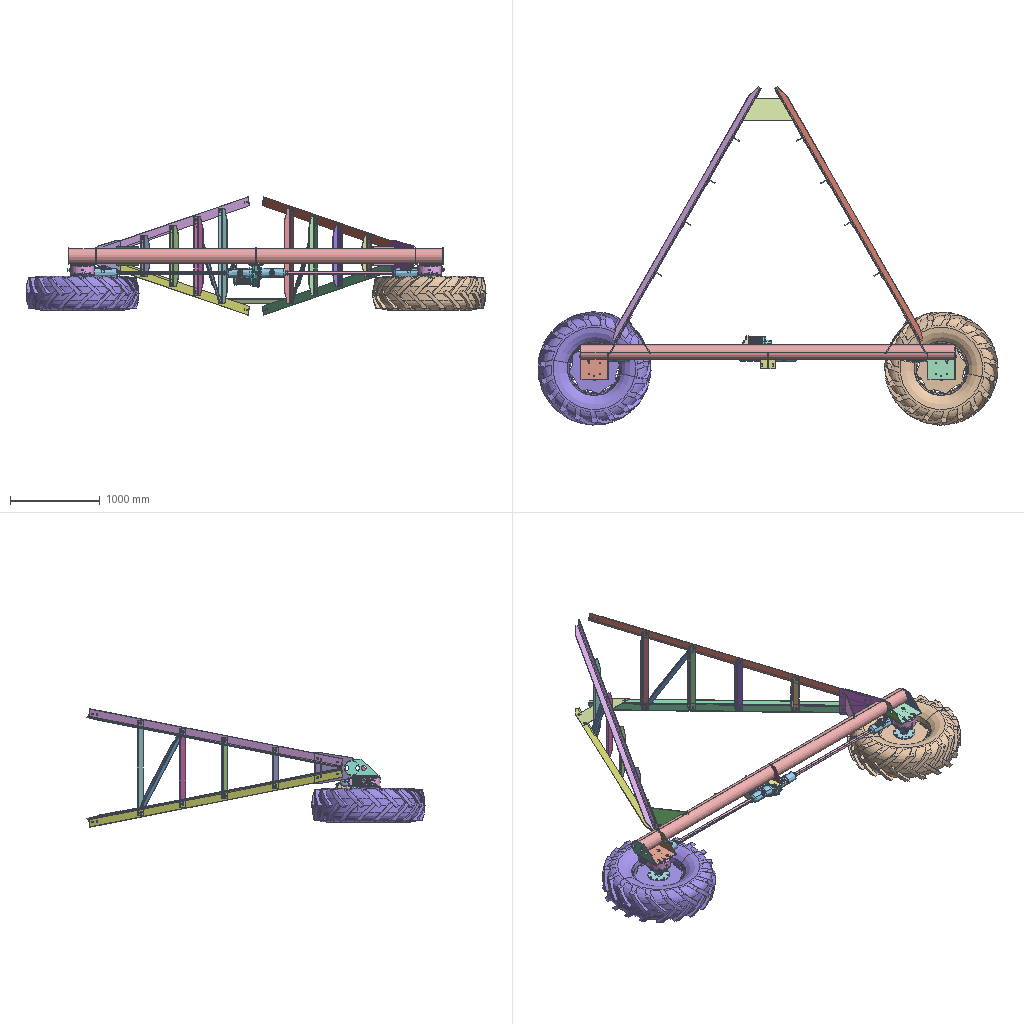Assembly | SolidWorks | 30 different items | 51 placed | box 5131 x 3771 x 1320 mm
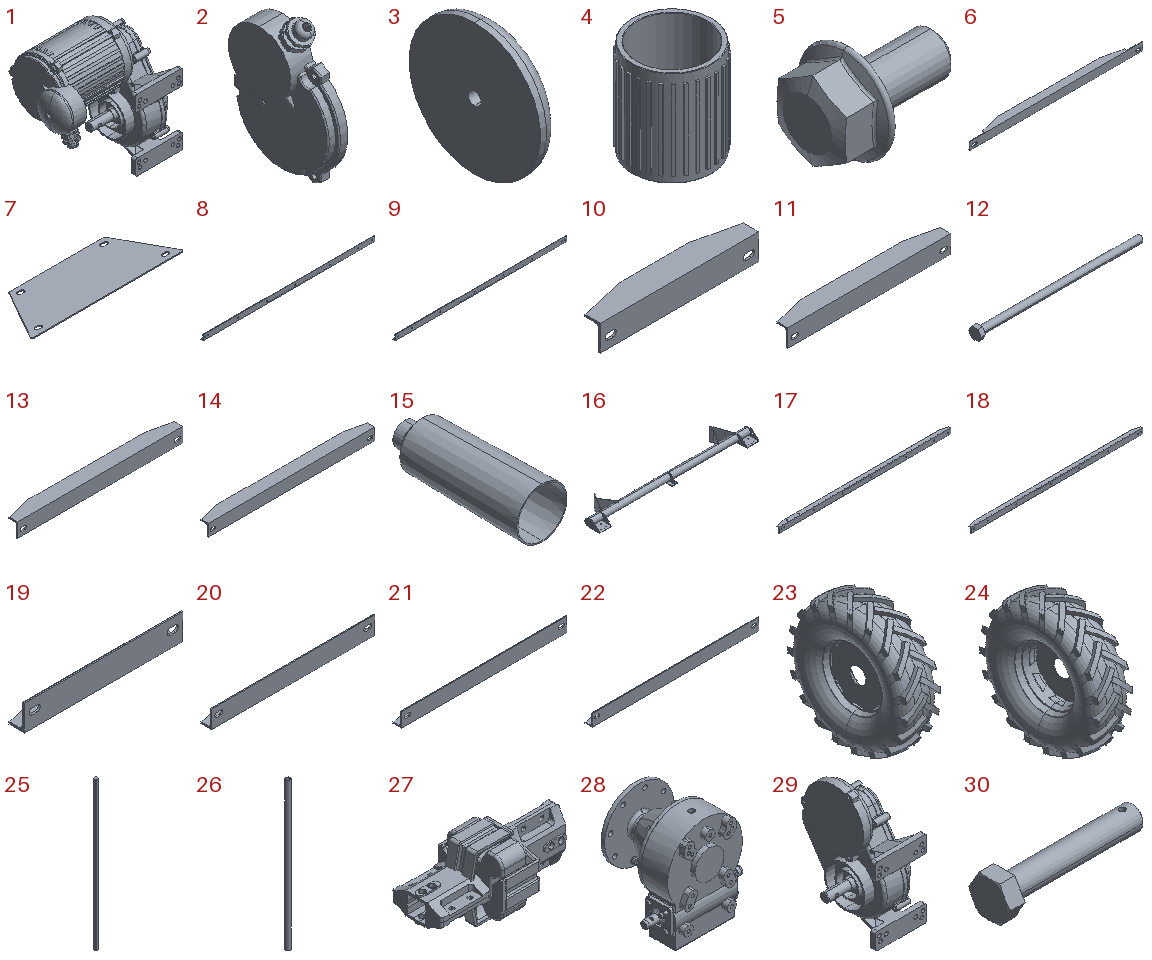Parts list (item | name | quantity | parent item | size | volume | features):
1 | (subassembly) | x1 | - | 419.954 x 256.191 x 342.427 mm | 6353002 mm3 | -
2 | - | x1 | in 1 | 39.9 x 182.18 x 239.915 mm | 603976 mm3 | features BaseBody 1
3 | - | x1 | in 1 | 24.913 x 107.2 x 107.2 mm | 163511 mm3 | features BaseBody 1
4 | - | x1 | in 1 | 172.079 x 171.827 x 198 mm | 1054388 mm3 | features BaseBody 1
5 | - | x1 | in 1 | 24.1 x 18 x 18 mm | 2099 mm3 | features BaseBody 1
6 | - | x2 | - | 1113 x 50 x 50 mm | 463803 mm3 | features ICE 3, WeldMemberFeat 1, WeldmentFeature 1
7 | - | x1 | - | 737.939 x 250 x 5 mm | 745580 mm3 | features FlatPattern 1, SMBaseFlange 1, SheetMetal 1
8 | - | x2 | - | 3300 x 80 x 100 mm | 4536810 mm3 | features Chamfer 2, ICE 2, WeldMemberFeat 1, WeldmentFeature 1
9 | - | x2 | - | 3300 x 80 x 100 mm | 4540882 mm3 | features Chamfer 2, ICE 1, WeldMemberFeat 1, WeldmentFeature 1
10 | - | x1 | - | 462 x 75 x 75 mm | 376932 mm3 | features Chamfer 2, ICE 1, WeldMemberFeat 1, WeldmentFeature 1
11 | - | x1 | - | 686 x 75 x 75 mm | 573977 mm3 | features Chamfer 2, ICE 2, WeldMemberFeat 1, WeldmentFeature 1
12 | - | x3 | in 1 | 195.95 x 14.699 x 12.73 mm | 10367 mm3 | features BaseBody 1
13 | - | x1 | - | 871 x 75 x 75 mm | 736715 mm3 | features Chamfer 2, ICE 1, WeldMemberFeat 1, WeldmentFeature 1
14 | - | x1 | - | 1056 x 75 x 75 mm | 899453 mm3 | features Chamfer 2, ICE 1, WeldMemberFeat 1, WeldmentFeature 1
15 | - | x4 | - | 110 x 300 x 110 mm | 234806 mm3 | features Revolution 1, Shell 1
16 | - | x1 | - | 4180 x 717.634 x 350 mm | 12364755 mm3 | features ICE 11, Cut 3, Fillet 3, BossThin 2, Extrusion 1, MirrorSolid 1
17 | - | x1 | - | 3300 x 80 x 100 mm | 4536810 mm3 | features MirrorStock 1
18 | - | x1 | - | 3300 x 80 x 100 mm | 4540882 mm3 | features MirrorStock 1
19 | - | x1 | - | 462 x 75 x 75 mm | 376932 mm3 | features MirrorStock 1
20 | - | x1 | - | 686 x 75 x 75 mm | 573977 mm3 | features MirrorStock 1
21 | - | x1 | - | 871 x 75 x 75 mm | 736715 mm3 | features MirrorStock 1
22 | - | x1 | - | 1056 x 75 x 75 mm | 899453 mm3 | features MirrorStock 1
23 | - | x1 | - | 378 x 1264 x 1263 mm | 294316338 mm3 | features CirPattern 2, ICE 2, RevCut 2, Revolution 2, Fillet 1, MoveFace 1
24 | - | x1 | - | 378 x 1264 x 1263 mm | 294316372 mm3 | features CirPattern 2, ICE 2, RevCut 2, Revolution 2, Fillet 1, MoveFace 1
25 | - | x2 | - | 24 x 24 x 1440 mm | 829131 mm3 | features Extrusion 1
26 | - | x2 | - | 40 x 40 x 1300 mm | 453332 mm3 | features Extrusion 1
27 | - | x4 | - | - | - | features RefSurface 9
28 | - | x2 | - | 334 x 277.06 x 364.795 mm | 6574332 mm3 | features BaseBody 36
29 | - | x1 | in 1 | 251 x 256.191 x 342.363 mm | 4473281 mm3 | features BaseBody 1
30 | - | x8 | in 1 | 50.95 x 14.699 x 12.73 mm | 3053 mm3 | features BaseBody 1
Mates (type | each side: item.copy, entity, surface, feature):
Coincident | 16.1 face plane Mirror2 | assembly face
Width | assembly face | assembly face | 16.1 face plane Mirror2 | 16.1 face plane Mirror2
DistanceDim | assembly face | 16.1 face plane Mirror2
Coincident | 16.1 face plane Boss-Extrude4 | assembly face
Width | assembly face | assembly face | 16.1 face plane Boss-Extrude2 | 16.1 face plane Boss-Extrude3
Coincident | assembly face | assembly face
Coincident | 16.1 face plane Boss-Extrude5 | 29.1 face plane Input 1
Width | 29.1 face plane Input 1 | 29.1 face plane Input 1 | 16.1 face plane Boss-Extrude5 | 16.1 face plane Boss-Extrude5 | 2 times
Concentric | 29.1 face cylinder Input 1 | 27.1 face cylinder Aluminum sheet-4-surface1
Concentric | 29.1 face cylinder Input 1 | 27.1 face cylinder Aluminum sheet-3-surface1
Concentric | assembly face | 27.2 face cylinder Aluminum sheet-2-surface1
Concentric | 29.1 face cylinder Input 1 | 27.3 face cylinder Aluminum sheet-2-surface1
Concentric | 29.1 face cylinder Input 1 | 27.3 face cylinder Aluminum sheet-1-surface1
Concentric | assembly face | 27.4 face cylinder Aluminum sheet-3-surface1
Concentric | assembly face | 27.2 face cylinder Aluminum sheet-1-surface1
Concentric | assembly face | 27.4 face cylinder Aluminum sheet-4-surface1
Width | 25.1 face plane Boss-Extrude1 | 25.1 face plane Boss-Extrude1 | 27.1 face plane Aluminum sheet-1-surface1 | 27.1 face plane Aluminum sheet-1-surface1
Width | 25.1 face plane Boss-Extrude1 | 25.1 face plane Boss-Extrude1 | 27.1 face plane Aluminum sheet-2-surface1 | 27.1 face plane Aluminum sheet-1-surface1
DistanceDim | 25.1 face plane Boss-Extrude1 | 27.1 face plane Aluminum sheet-1-surface1
Width | 25.2 face plane Boss-Extrude1 | 25.2 face plane Boss-Extrude1 | 27.3 face plane Aluminum sheet-4-surface1 | 27.3 face plane Aluminum sheet-3-surface1
Width | 25.2 face plane Boss-Extrude1 | 25.2 face plane Boss-Extrude1 | 27.3 face plane Aluminum sheet-3-surface1 | 27.3 face plane Aluminum sheet-3-surface1
DistanceDim | 25.2 face plane Boss-Extrude1 | 27.3 face plane Aluminum sheet-4-surface1
Concentric | 29.1 face cylinder Input 1 | 26.1 face cylinder Boss-Extrude1
Width | 26.1 face plane Boss-Extrude1 | 26.1 face plane Boss-Extrude1 | 27.1 face plane Aluminum sheet-1-surface1 | 27.2 face plane Aluminum sheet-4-surface1
Concentric | 29.1 face cylinder Input 1 | 26.2 face cylinder Boss-Extrude1
Width | 26.2 face plane Boss-Extrude1 | 26.2 face plane Boss-Extrude1 | 27.4 face plane Aluminum sheet-2-surface1 | 27.3 face plane Aluminum sheet-4-surface1
Concentric | 26.1 face cylinder Boss-Extrude1 | 15.1 face cylinder Shell1
Concentric | 26.1 face cylinder Boss-Extrude1 | 15.2 face cylinder Shell1
Concentric | 26.2 face cylinder Boss-Extrude1 | 15.3 face cylinder Shell1
Concentric | 26.2 face cylinder Boss-Extrude1 | 15.4 face cylinder Revolve1
Concentric | assembly face | 23.1 face cylinder Revolve3
Concentric | assembly face | 23.1 face cylinder Cut-Extrude1
Coincident | assembly face | 23.1 face plane Revolve3
Concentric | assembly face | 24.1 face cylinder Revolve3
Concentric | assembly face | 24.1 face cylinder Cut-Extrude1
Coincident | assembly face | 24.1 face plane Revolve3
Coincident | 16.1 face plane Mirror2 | 8.1 face plane Hot-rolled unequal-leg angle steel (gb t9788-1988) 100×80×8(1)
Concentric | 16.1 face cylinder Mirror2 | 8.1 face cylinder Cut-Extrude1 | 2 times
Concentric | 16.1 face cylinder Mirror2 | 9.1 face cylinder Cut-Extrude1 | 2 times
Coincident | 16.1 face plane Mirror2 | 9.1 face plane Hot-rolled unequal-leg angle steel (gb t9788-1988) 100×80×8(1)
Concentric | 8.1 face cylinder Cut-Extrude1 | 10.1 select_type:25
Coincident | 8.1 face plane Hot-rolled unequal-leg angle steel (gb t9788-1988) 100×80×8(1) | 10.1 face plane Hot-rolled equal-leg angle steel (gb t9787-1988) 75×6(1)
Concentric | 8.1 face cylinder Cut-Extrude1 | 11.1 select_type:25
Coincident | 8.1 face plane Hot-rolled unequal-leg angle steel (gb t9788-1988) 100×80×8(1) | 11.1 face plane Hot-rolled equal-leg angle steel (gb t9787-1988) 75×6(1)
Concentric | 8.1 face cylinder Cut-Extrude1 | 13.1 select_type:25
Coincident | 8.1 face plane Hot-rolled unequal-leg angle steel (gb t9788-1988) 100×80×8(1) | 13.1 face plane Hot-rolled equal-leg angle steel (gb t9787-1988) 75×6(1)
Concentric | 8.1 face cylinder Cut-Extrude1 | 14.1 select_type:25
Coincident | 8.1 face plane Hot-rolled unequal-leg angle steel (gb t9788-1988) 100×80×8(1) | 14.1 face plane Hot-rolled equal-leg angle steel (gb t9787-1988) 75×6(1)
Coincident | 11.1 face plane Hot-rolled equal-leg angle steel (gb t9787-1988) 75×6(1) | assembly face
Concentric | 11.1 face | assembly face | 2 times
Concentric | 16.1 face cylinder Cut-Extrude4 | 28.1 face cylinder | 2 times
Coincident | 16.1 face plane Mirror2 | 28.1 face plane
Concentric | 28.1 face cylinder | 23.1 face cylinder Revolve3
Concentric | 28.1 face cylinder hex flange bolt_is_IS 15582 - M10 x 20 x 20-N.STEP.STEP-17-solid1 | 23.1 face cylinder Cut-Extrude1
Coincident | 28.1 face plane | 23.1 face plane Revolve3
Concentric | 16.1 face cylinder Cut-Extrude3 | 28.2 face cylinder | 2 times
Coincident | 16.1 face plane Boss-Extrude4 | 28.2 face plane
Concentric | 28.2 face cylinder | 24.1 face cylinder Revolve3
Concentric | 28.2 face cylinder hex flange bolt_is_IS 15582 - M10 x 20 x 20-N.STEP.STEP-17-solid1 | 24.1 face cylinder Cut-Extrude1
Coincident | 28.2 face plane | 24.1 face plane Revolve3
Concentric | 16.1 face cylinder Mirror2 | 9.2 face cylinder Cut-Extrude1 | 2 times
Coincident | 16.1 face plane Mirror2 | 9.2 face plane Hot-rolled unequal-leg angle steel (gb t9788-1988) 100×80×8(1)
Concentric | 16.1 face cylinder Mirror2 | 8.2 face cylinder Cut-Extrude1 | 2 times
Coincident | 16.1 face plane Mirror2 | 8.2 face plane Hot-rolled unequal-leg angle steel (gb t9788-1988) 100×80×8(1)
Coincident | 13.1 face plane Hot-rolled equal-leg angle steel (gb t9787-1988) 75×6(1) | 6.1 face plane Hot-rolled equal-leg angle steel (gb t9787-1988) 50×5(1)
Slot | 6.1 face plane Cut-Extrude1 | 9.1 face cylinder Cut-Extrude1
Coincident | 13.1 face plane Hot-rolled equal-leg angle steel (gb t9787-1988) 75×6(1) | assembly face | 2 times
Slot | assembly face | 9.1 face cylinder Cut-Extrude1 | 2 times
Parallel | 8.1 select_type:24 | 7.1 face plane Base-Flange1
Parallel | 16.1 face plane Boss-Extrude7 | 7.1 edge